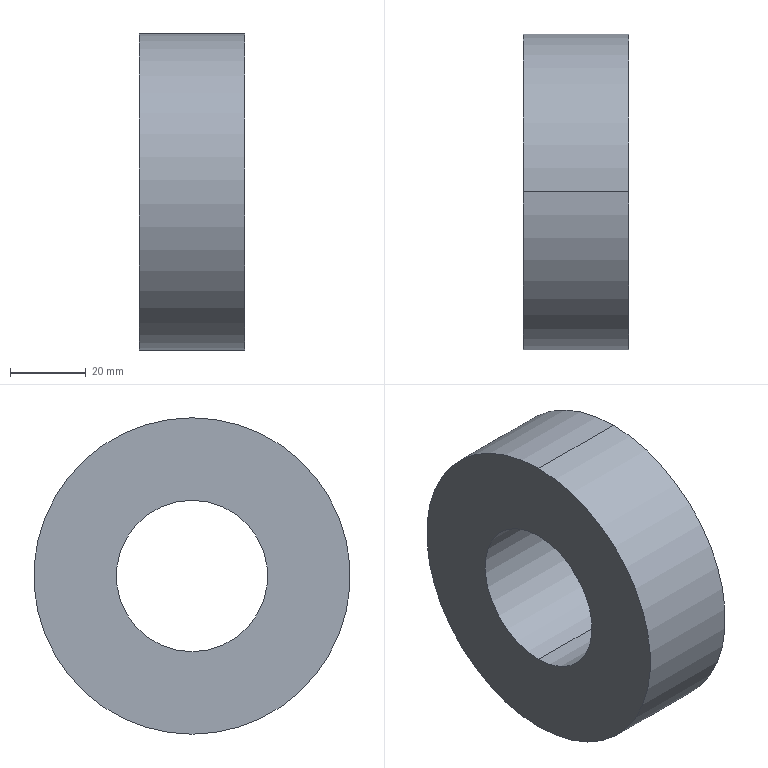Part | SolidWorks | features Extrusion 1 | 1 solid | 6 faces | box 28 x 83.6 x 83.6 mm | volume 118509 mm3 | cylinder 4 | plane 2 | commonest cylinder face diameters 40 x2 83.6 x2
STEP:
#1=CARTESIAN_POINT('',(28.,0.,20.));
#2=VERTEX_POINT('',#1);
#3=CARTESIAN_POINT('',(28.,0.,-20.));
#4=VERTEX_POINT('',#3);
#5=CARTESIAN_POINT('',(28.,0.,0.));
#6=DIRECTION('',(1.,0.,0.));
#7=DIRECTION('',(0.,0.,-1.));
#8=AXIS2_PLACEMENT_3D('',#5,#6,#7);
#9=CIRCLE('',#8,20.);
#10=EDGE_CURVE('',#2,#4,#9,.T.);
#11=ORIENTED_EDGE('',*,*,#10,.T.);
#12=CARTESIAN_POINT('',(0.,0.,-20.));
#13=VERTEX_POINT('',#12);
#14=CARTESIAN_POINT('',(28.,0.,-20.));
#15=DIRECTION('',(-1.,0.,0.));
#16=VECTOR('',#15,1000.);
#17=LINE('',#14,#16);
#18=EDGE_CURVE('',#4,#13,#17,.T.);
#19=ORIENTED_EDGE('',*,*,#18,.T.);
#20=CARTESIAN_POINT('',(0.,0.,20.));
#21=VERTEX_POINT('',#20);
#22=CARTESIAN_POINT('',(0.,0.,0.));
#23=DIRECTION('',(1.,0.,0.));
#24=DIRECTION('',(0.,0.,-1.));
#25=AXIS2_PLACEMENT_3D('',#22,#23,#24);
#26=CIRCLE('',#25,20.);
#27=EDGE_CURVE('',#21,#13,#26,.T.);
#28=ORIENTED_EDGE('',*,*,#27,.F.);
#29=CARTESIAN_POINT('',(28.,0.,20.));
#30=DIRECTION('',(-1.,0.,0.));
#31=VECTOR('',#30,1000.);
#32=LINE('',#29,#31);
#33=EDGE_CURVE('',#2,#21,#32,.T.);
#34=ORIENTED_EDGE('',*,*,#33,.F.);
#35=EDGE_LOOP('',(#11,#19,#28,#34));
#36=FACE_OUTER_BOUND('',#35,.T.);
#37=CARTESIAN_POINT('',(28.,0.,0.));
#38=DIRECTION('',(-1.,0.,0.));
#39=DIRECTION('',(0.,0.,1.));
#40=AXIS2_PLACEMENT_3D('',#37,#38,#39);
#41=CYLINDRICAL_SURFACE('',#40,20.);
#42=ADVANCED_FACE('',(#36),#41,.F.);
#43=CARTESIAN_POINT('',(28.,0.,-41.8));
#44=VERTEX_POINT('',#43);
#45=CARTESIAN_POINT('',(28.,0.,41.8));
#46=VERTEX_POINT('',#45);
#47=CARTESIAN_POINT('',(28.,0.,0.));
#48=DIRECTION('',(1.,0.,0.));
#49=DIRECTION('',(0.,0.,-1.));
#50=AXIS2_PLACEMENT_3D('',#47,#48,#49);
#51=CIRCLE('',#50,41.8);
#52=EDGE_CURVE('',#44,#46,#51,.T.);
#53=ORIENTED_EDGE('',*,*,#52,.F.);
#54=CARTESIAN_POINT('',(0.,0.,-41.8));
#55=VERTEX_POINT('',#54);
#56=CARTESIAN_POINT('',(28.,0.,-41.8));
#57=DIRECTION('',(-1.,0.,0.));
#58=VECTOR('',#57,1000.);
#59=LINE('',#56,#58);
#60=EDGE_CURVE('',#44,#55,#59,.T.);
#61=ORIENTED_EDGE('',*,*,#60,.T.);
#62=CARTESIAN_POINT('',(0.,0.,41.8));
#63=VERTEX_POINT('',#62);
#64=CARTESIAN_POINT('',(0.,0.,0.));
#65=DIRECTION('',(1.,0.,0.));
#66=DIRECTION('',(0.,0.,-1.));
#67=AXIS2_PLACEMENT_3D('',#64,#65,#66);
#68=CIRCLE('',#67,41.8);
#69=EDGE_CURVE('',#55,#63,#68,.T.);
#70=ORIENTED_EDGE('',*,*,#69,.T.);
#71=CARTESIAN_POINT('',(28.,0.,41.8));
#72=DIRECTION('',(-1.,0.,0.));
#73=VECTOR('',#72,1000.);
#74=LINE('',#71,#73);
#75=EDGE_CURVE('',#46,#63,#74,.T.);
#76=ORIENTED_EDGE('',*,*,#75,.F.);
#77=EDGE_LOOP('',(#53,#61,#70,#76));
#78=FACE_OUTER_BOUND('',#77,.T.);
#79=CARTESIAN_POINT('',(28.,0.,0.));
#80=DIRECTION('',(-1.,0.,0.));
#81=DIRECTION('',(0.,0.,1.));
#82=AXIS2_PLACEMENT_3D('',#79,#80,#81);
#83=CYLINDRICAL_SURFACE('',#82,41.8);
#84=ADVANCED_FACE('',(#78),#83,.T.);
#85=CARTESIAN_POINT('',(28.,0.,0.));
#86=DIRECTION('',(1.,0.,0.));
#87=DIRECTION('',(0.,0.,-1.));
#88=AXIS2_PLACEMENT_3D('',#85,#86,#87);
#89=CIRCLE('',#88,41.8);
#90=EDGE_CURVE('',#46,#44,#89,.T.);
#91=ORIENTED_EDGE('',*,*,#90,.T.);
#92=ORIENTED_EDGE('',*,*,#52,.T.);
#93=EDGE_LOOP('',(#91,#92));
#94=FACE_OUTER_BOUND('',#93,.T.);
#95=ORIENTED_EDGE('',*,*,#10,.F.);
#96=CARTESIAN_POINT('',(28.,0.,0.));
#97=DIRECTION('',(1.,0.,0.));
#98=DIRECTION('',(0.,0.,-1.));
#99=AXIS2_PLACEMENT_3D('',#96,#97,#98);
#100=CIRCLE('',#99,20.);
#101=EDGE_CURVE('',#4,#2,#100,.T.);
#102=ORIENTED_EDGE('',*,*,#101,.F.);
#103=EDGE_LOOP('',(#95,#102));
#104=FACE_BOUND('',#103,.T.);
#105=CARTESIAN_POINT('',(28.,0.,0.));
#106=DIRECTION('',(1.,0.,0.));
#107=DIRECTION('',(0.,0.,-1.));
#108=AXIS2_PLACEMENT_3D('',#105,#106,#107);
#109=PLANE('',#108);
#110=ADVANCED_FACE('',(#94,#104),#109,.T.);
#111=CARTESIAN_POINT('',(0.,0.,0.));
#112=DIRECTION('',(1.,0.,0.));
#113=DIRECTION('',(0.,0.,-1.));
#114=AXIS2_PLACEMENT_3D('',#111,#112,#113);
#115=CIRCLE('',#114,41.8);
#116=EDGE_CURVE('',#63,#55,#115,.T.);
#117=ORIENTED_EDGE('',*,*,#116,.F.);
#118=ORIENTED_EDGE('',*,*,#69,.F.);
#119=EDGE_LOOP('',(#117,#118));
#120=FACE_OUTER_BOUND('',#119,.T.);
#121=ORIENTED_EDGE('',*,*,#27,.T.);
#122=CARTESIAN_POINT('',(0.,0.,0.));
#123=DIRECTION('',(1.,0.,0.));
#124=DIRECTION('',(0.,0.,-1.));
#125=AXIS2_PLACEMENT_3D('',#122,#123,#124);
#126=CIRCLE('',#125,20.);
#127=EDGE_CURVE('',#13,#21,#126,.T.);
#128=ORIENTED_EDGE('',*,*,#127,.T.);
#129=EDGE_LOOP('',(#121,#128));
#130=FACE_BOUND('',#129,.T.);
#131=CARTESIAN_POINT('',(0.,0.,0.));
#132=DIRECTION('',(1.,0.,0.));
#133=DIRECTION('',(0.,0.,-1.));
#134=AXIS2_PLACEMENT_3D('',#131,#132,#133);
#135=PLANE('',#134);
#136=ADVANCED_FACE('',(#120,#130),#135,.F.);
#137=ORIENTED_EDGE('',*,*,#60,.F.);
#138=ORIENTED_EDGE('',*,*,#90,.F.);
#139=ORIENTED_EDGE('',*,*,#75,.T.);
#140=ORIENTED_EDGE('',*,*,#116,.T.);
#141=EDGE_LOOP('',(#137,#138,#139,#140));
#142=FACE_OUTER_BOUND('',#141,.T.);
#143=CARTESIAN_POINT('',(28.,0.,0.));
#144=DIRECTION('',(-1.,0.,0.));
#145=DIRECTION('',(0.,0.,1.));
#146=AXIS2_PLACEMENT_3D('',#143,#144,#145);
#147=CYLINDRICAL_SURFACE('',#146,41.8);
#148=ADVANCED_FACE('',(#142),#147,.T.);
#149=ORIENTED_EDGE('',*,*,#18,.F.);
#150=ORIENTED_EDGE('',*,*,#101,.T.);
#151=ORIENTED_EDGE('',*,*,#33,.T.);
#152=ORIENTED_EDGE('',*,*,#127,.F.);
#153=EDGE_LOOP('',(#149,#150,#151,#152));
#154=FACE_OUTER_BOUND('',#153,.T.);
#155=CARTESIAN_POINT('',(28.,0.,0.));
#156=DIRECTION('',(-1.,0.,0.));
#157=DIRECTION('',(0.,0.,1.));
#158=AXIS2_PLACEMENT_3D('',#155,#156,#157);
#159=CYLINDRICAL_SURFACE('',#158,20.);
#160=ADVANCED_FACE('',(#154),#159,.F.);
#161=CLOSED_SHELL('',(#42,#84,#110,#136,#148,#160));
#162=MANIFOLD_SOLID_BREP('',#161);
#163=CARTESIAN_POINT('',(0.,0.,0.));
#164=DIRECTION('',(0.,0.,1.));
#165=DIRECTION('',(1.,0.,0.));
#166=AXIS2_PLACEMENT_3D('',#163,#164,#165);
#167=(LENGTH_UNIT()NAMED_UNIT(*)SI_UNIT(.MILLI.,.METRE.));
#168=UNCERTAINTY_MEASURE_WITH_UNIT(LENGTH_MEASURE(0.00001),#167,'','');
#169=(NAMED_UNIT(*)PLANE_ANGLE_UNIT()SI_UNIT($,.RADIAN.));
#170=(NAMED_UNIT(*)SI_UNIT($,.STERADIAN.)SOLID_ANGLE_UNIT());
#171=(GEOMETRIC_REPRESENTATION_CONTEXT(3)GLOBAL_UNCERTAINTY_ASSIGNED_CONTEXT((#168))GLOBAL_UNIT_ASSIGNED_CONTEXT((#167,#169,#170))REPRESENTATION_CONTEXT('',''));
#172=ADVANCED_BREP_SHAPE_REPRESENTATION('',(#162,#166),#171);